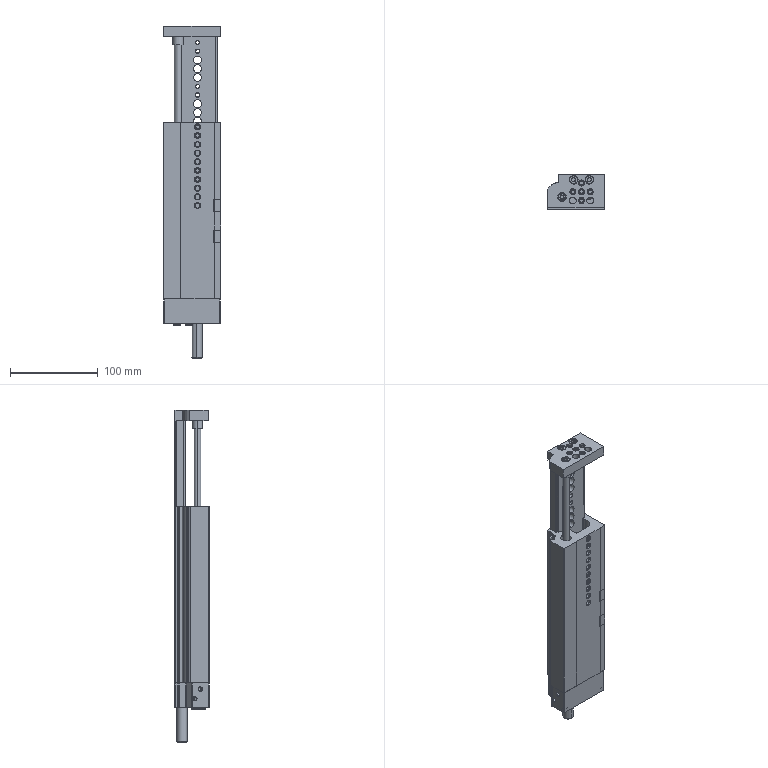Part | SolidWorks | 8 solids | 852 faces | box 66 x 40 x 379 mm | volume 460415 mm3 | plane 372 | cylinder 322 | cone 144 | torus 14 | commonest cylinder face diameters 7 x46 0.4 x39 4.134 x39 8 x24 9 x24 10 x24